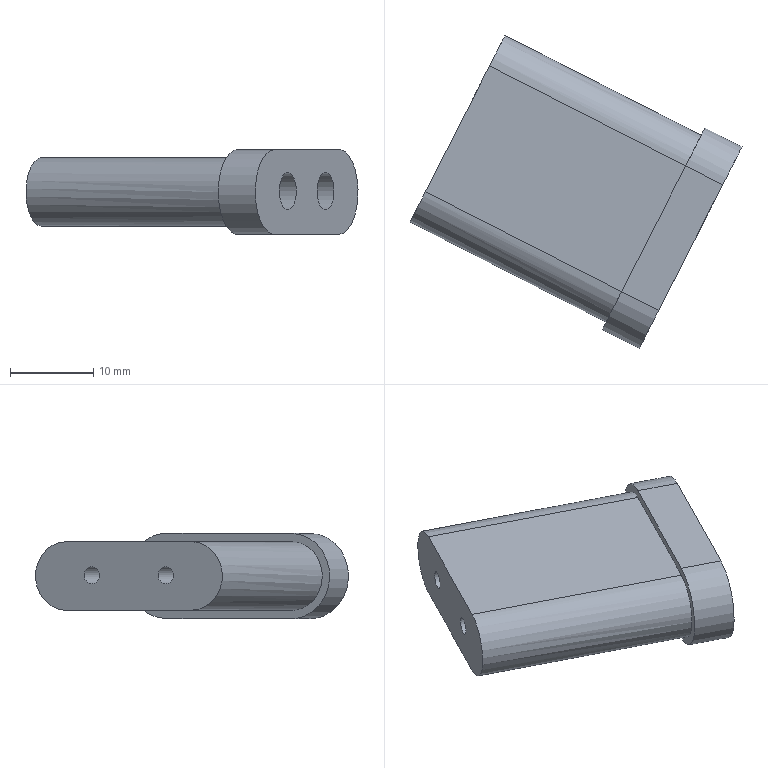Part | STEP file | gslz 2016.10.28-13_id66_x_t | 1 solid | 17 faces | box 39.984 x 37.689 x 10.246 mm | volume 5772 mm3 | plane 9 | spline 4 | cylinder 4 | commonest cylinder face diameters 2.1 x2 4.5 x2